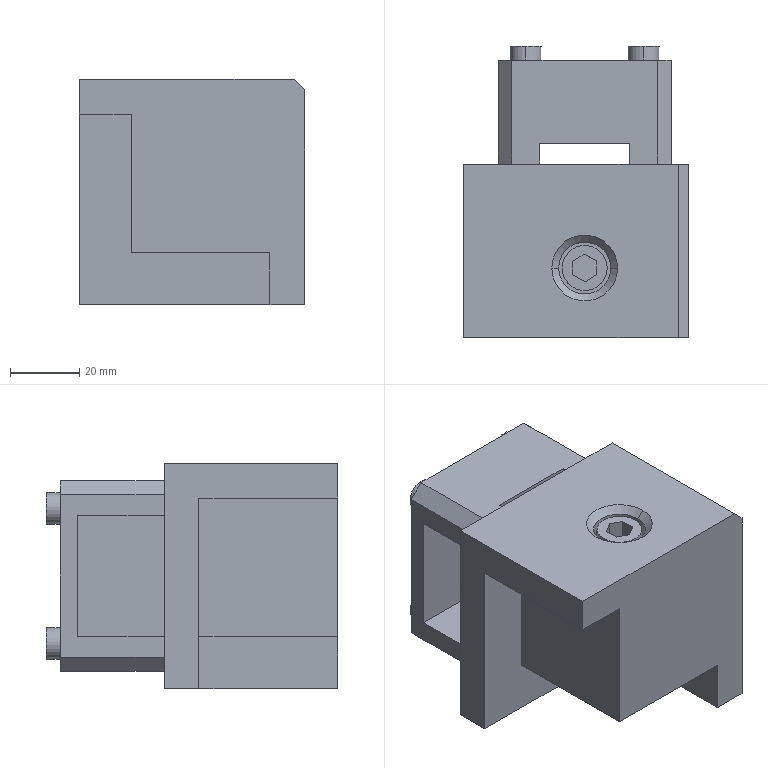Part | SolidWorks | features ICE 10, Chamfer 3, Extrusion 1 | 1 solid | 101 faces | box 65 x 84 x 65 mm | volume 191550 mm3 | plane 81 | cylinder 16 | cone 4 | commonest cylinder face diameters 9 x8 13 x4 15 x4